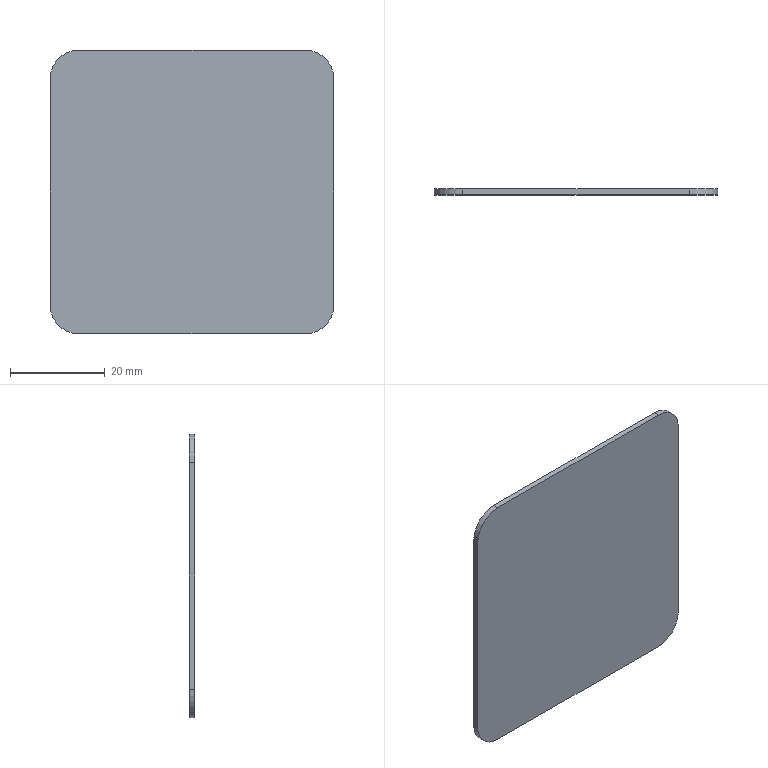Part | STEP file | JBJ-P-1017-02 | 1 solid | 10 faces | box 60 x 1.2 x 60 mm | volume 4283 mm3 | plane 6 | cylinder 4 | commonest cylinder face diameters 12 x4
STEP:
#1=CARTESIAN_POINT('',(30.,0.,-24.));
#2=VERTEX_POINT('',#1);
#3=CARTESIAN_POINT('',(24.,0.,-30.));
#4=VERTEX_POINT('',#3);
#5=CARTESIAN_POINT('',(24.,0.,-24.));
#6=DIRECTION('',(0.,1.,0.));
#7=DIRECTION('',(0.,0.,-1.));
#8=AXIS2_PLACEMENT_3D('',#5,#6,#7);
#9=CIRCLE('',#8,6.);
#10=EDGE_CURVE('',#2,#4,#9,.T.);
#11=ORIENTED_EDGE('',*,*,#10,.T.);
#12=CARTESIAN_POINT('',(24.,1.2,-30.));
#13=VERTEX_POINT('',#12);
#14=CARTESIAN_POINT('',(24.,1.2,-30.));
#15=DIRECTION('',(0.,-1.,0.));
#16=VECTOR('',#15,1000.);
#17=LINE('',#14,#16);
#18=EDGE_CURVE('',#13,#4,#17,.T.);
#19=ORIENTED_EDGE('',*,*,#18,.F.);
#20=CARTESIAN_POINT('',(30.,1.2,-24.));
#21=VERTEX_POINT('',#20);
#22=CARTESIAN_POINT('',(24.,1.2,-24.));
#23=DIRECTION('',(0.,1.,0.));
#24=DIRECTION('',(0.,0.,-1.));
#25=AXIS2_PLACEMENT_3D('',#22,#23,#24);
#26=CIRCLE('',#25,6.);
#27=EDGE_CURVE('',#21,#13,#26,.T.);
#28=ORIENTED_EDGE('',*,*,#27,.F.);
#29=CARTESIAN_POINT('',(30.,1.2,-24.));
#30=DIRECTION('',(0.,-1.,0.));
#31=VECTOR('',#30,1000.);
#32=LINE('',#29,#31);
#33=EDGE_CURVE('',#21,#2,#32,.T.);
#34=ORIENTED_EDGE('',*,*,#33,.T.);
#35=EDGE_LOOP('',(#11,#19,#28,#34));
#36=FACE_OUTER_BOUND('',#35,.T.);
#37=CARTESIAN_POINT('',(24.,1.2,-24.));
#38=DIRECTION('',(0.,-1.,0.));
#39=DIRECTION('',(0.,0.,-1.));
#40=AXIS2_PLACEMENT_3D('',#37,#38,#39);
#41=CYLINDRICAL_SURFACE('',#40,6.);
#42=ADVANCED_FACE('',(#36),#41,.T.);
#43=CARTESIAN_POINT('',(-24.,0.,-30.));
#44=VERTEX_POINT('',#43);
#45=CARTESIAN_POINT('',(-24.,0.,-30.));
#46=DIRECTION('',(-1.,0.,0.));
#47=VECTOR('',#46,1000.);
#48=LINE('',#45,#47);
#49=EDGE_CURVE('',#4,#44,#48,.T.);
#50=ORIENTED_EDGE('',*,*,#49,.T.);
#51=CARTESIAN_POINT('',(-24.,1.2,-30.));
#52=VERTEX_POINT('',#51);
#53=CARTESIAN_POINT('',(-24.,1.2,-30.));
#54=DIRECTION('',(0.,-1.,0.));
#55=VECTOR('',#54,1000.);
#56=LINE('',#53,#55);
#57=EDGE_CURVE('',#52,#44,#56,.T.);
#58=ORIENTED_EDGE('',*,*,#57,.F.);
#59=CARTESIAN_POINT('',(-24.,1.2,-30.));
#60=DIRECTION('',(-1.,0.,0.));
#61=VECTOR('',#60,1000.);
#62=LINE('',#59,#61);
#63=EDGE_CURVE('',#13,#52,#62,.T.);
#64=ORIENTED_EDGE('',*,*,#63,.F.);
#65=ORIENTED_EDGE('',*,*,#18,.T.);
#66=EDGE_LOOP('',(#50,#58,#64,#65));
#67=FACE_OUTER_BOUND('',#66,.T.);
#68=CARTESIAN_POINT('',(-24.,1.2,-30.));
#69=DIRECTION('',(0.,0.,1.));
#70=DIRECTION('',(1.,0.,0.));
#71=AXIS2_PLACEMENT_3D('',#68,#69,#70);
#72=PLANE('',#71);
#73=ADVANCED_FACE('',(#67),#72,.F.);
#74=CARTESIAN_POINT('',(-30.,0.,-24.));
#75=VERTEX_POINT('',#74);
#76=CARTESIAN_POINT('',(-24.,0.,-24.));
#77=DIRECTION('',(0.,1.,0.));
#78=DIRECTION('',(0.,0.,1.));
#79=AXIS2_PLACEMENT_3D('',#76,#77,#78);
#80=CIRCLE('',#79,6.);
#81=EDGE_CURVE('',#44,#75,#80,.T.);
#82=ORIENTED_EDGE('',*,*,#81,.T.);
#83=CARTESIAN_POINT('',(-30.,1.2,-24.));
#84=VERTEX_POINT('',#83);
#85=CARTESIAN_POINT('',(-30.,1.2,-24.));
#86=DIRECTION('',(0.,-1.,0.));
#87=VECTOR('',#86,1000.);
#88=LINE('',#85,#87);
#89=EDGE_CURVE('',#84,#75,#88,.T.);
#90=ORIENTED_EDGE('',*,*,#89,.F.);
#91=CARTESIAN_POINT('',(-24.,1.2,-24.));
#92=DIRECTION('',(0.,1.,0.));
#93=DIRECTION('',(0.,0.,1.));
#94=AXIS2_PLACEMENT_3D('',#91,#92,#93);
#95=CIRCLE('',#94,6.);
#96=EDGE_CURVE('',#52,#84,#95,.T.);
#97=ORIENTED_EDGE('',*,*,#96,.F.);
#98=ORIENTED_EDGE('',*,*,#57,.T.);
#99=EDGE_LOOP('',(#82,#90,#97,#98));
#100=FACE_OUTER_BOUND('',#99,.T.);
#101=CARTESIAN_POINT('',(-24.,1.2,-24.));
#102=DIRECTION('',(0.,-1.,0.));
#103=DIRECTION('',(0.,0.,-1.));
#104=AXIS2_PLACEMENT_3D('',#101,#102,#103);
#105=CYLINDRICAL_SURFACE('',#104,6.);
#106=ADVANCED_FACE('',(#100),#105,.T.);
#107=CARTESIAN_POINT('',(-30.,0.,24.));
#108=VERTEX_POINT('',#107);
#109=CARTESIAN_POINT('',(-30.,0.,-24.));
#110=DIRECTION('',(0.,0.,1.));
#111=VECTOR('',#110,1000.);
#112=LINE('',#109,#111);
#113=EDGE_CURVE('',#75,#108,#112,.T.);
#114=ORIENTED_EDGE('',*,*,#113,.T.);
#115=CARTESIAN_POINT('',(-30.,1.2,24.));
#116=VERTEX_POINT('',#115);
#117=CARTESIAN_POINT('',(-30.,1.2,24.));
#118=DIRECTION('',(0.,-1.,0.));
#119=VECTOR('',#118,1000.);
#120=LINE('',#117,#119);
#121=EDGE_CURVE('',#116,#108,#120,.T.);
#122=ORIENTED_EDGE('',*,*,#121,.F.);
#123=CARTESIAN_POINT('',(-30.,1.2,-24.));
#124=DIRECTION('',(0.,0.,1.));
#125=VECTOR('',#124,1000.);
#126=LINE('',#123,#125);
#127=EDGE_CURVE('',#84,#116,#126,.T.);
#128=ORIENTED_EDGE('',*,*,#127,.F.);
#129=ORIENTED_EDGE('',*,*,#89,.T.);
#130=EDGE_LOOP('',(#114,#122,#128,#129));
#131=FACE_OUTER_BOUND('',#130,.T.);
#132=CARTESIAN_POINT('',(-30.,1.2,-24.));
#133=DIRECTION('',(1.,0.,0.));
#134=DIRECTION('',(0.,0.,-1.));
#135=AXIS2_PLACEMENT_3D('',#132,#133,#134);
#136=PLANE('',#135);
#137=ADVANCED_FACE('',(#131),#136,.F.);
#138=CARTESIAN_POINT('',(-24.,0.,30.));
#139=VERTEX_POINT('',#138);
#140=CARTESIAN_POINT('',(-24.,0.,24.));
#141=DIRECTION('',(0.,1.,0.));
#142=DIRECTION('',(0.,0.,1.));
#143=AXIS2_PLACEMENT_3D('',#140,#141,#142);
#144=CIRCLE('',#143,6.);
#145=EDGE_CURVE('',#108,#139,#144,.T.);
#146=ORIENTED_EDGE('',*,*,#145,.T.);
#147=CARTESIAN_POINT('',(-24.,1.2,30.));
#148=VERTEX_POINT('',#147);
#149=CARTESIAN_POINT('',(-24.,1.2,30.));
#150=DIRECTION('',(0.,-1.,0.));
#151=VECTOR('',#150,1000.);
#152=LINE('',#149,#151);
#153=EDGE_CURVE('',#148,#139,#152,.T.);
#154=ORIENTED_EDGE('',*,*,#153,.F.);
#155=CARTESIAN_POINT('',(-24.,1.2,24.));
#156=DIRECTION('',(0.,1.,0.));
#157=DIRECTION('',(0.,0.,1.));
#158=AXIS2_PLACEMENT_3D('',#155,#156,#157);
#159=CIRCLE('',#158,6.);
#160=EDGE_CURVE('',#116,#148,#159,.T.);
#161=ORIENTED_EDGE('',*,*,#160,.F.);
#162=ORIENTED_EDGE('',*,*,#121,.T.);
#163=EDGE_LOOP('',(#146,#154,#161,#162));
#164=FACE_OUTER_BOUND('',#163,.T.);
#165=CARTESIAN_POINT('',(-24.,1.2,24.));
#166=DIRECTION('',(0.,-1.,0.));
#167=DIRECTION('',(0.,0.,-1.));
#168=AXIS2_PLACEMENT_3D('',#165,#166,#167);
#169=CYLINDRICAL_SURFACE('',#168,6.);
#170=ADVANCED_FACE('',(#164),#169,.T.);
#171=CARTESIAN_POINT('',(24.,0.,30.));
#172=VERTEX_POINT('',#171);
#173=CARTESIAN_POINT('',(-24.,0.,30.));
#174=DIRECTION('',(1.,0.,0.));
#175=VECTOR('',#174,1000.);
#176=LINE('',#173,#175);
#177=EDGE_CURVE('',#139,#172,#176,.T.);
#178=ORIENTED_EDGE('',*,*,#177,.T.);
#179=CARTESIAN_POINT('',(24.,1.2,30.));
#180=VERTEX_POINT('',#179);
#181=CARTESIAN_POINT('',(24.,1.2,30.));
#182=DIRECTION('',(0.,-1.,0.));
#183=VECTOR('',#182,1000.);
#184=LINE('',#181,#183);
#185=EDGE_CURVE('',#180,#172,#184,.T.);
#186=ORIENTED_EDGE('',*,*,#185,.F.);
#187=CARTESIAN_POINT('',(-24.,1.2,30.));
#188=DIRECTION('',(1.,0.,0.));
#189=VECTOR('',#188,1000.);
#190=LINE('',#187,#189);
#191=EDGE_CURVE('',#148,#180,#190,.T.);
#192=ORIENTED_EDGE('',*,*,#191,.F.);
#193=ORIENTED_EDGE('',*,*,#153,.T.);
#194=EDGE_LOOP('',(#178,#186,#192,#193));
#195=FACE_OUTER_BOUND('',#194,.T.);
#196=CARTESIAN_POINT('',(-24.,1.2,30.));
#197=DIRECTION('',(0.,0.,-1.));
#198=DIRECTION('',(-1.,0.,0.));
#199=AXIS2_PLACEMENT_3D('',#196,#197,#198);
#200=PLANE('',#199);
#201=ADVANCED_FACE('',(#195),#200,.F.);
#202=CARTESIAN_POINT('',(30.,0.,24.));
#203=VERTEX_POINT('',#202);
#204=CARTESIAN_POINT('',(24.,0.,24.));
#205=DIRECTION('',(0.,1.,0.));
#206=DIRECTION('',(0.,0.,1.));
#207=AXIS2_PLACEMENT_3D('',#204,#205,#206);
#208=CIRCLE('',#207,6.);
#209=EDGE_CURVE('',#172,#203,#208,.T.);
#210=ORIENTED_EDGE('',*,*,#209,.T.);
#211=CARTESIAN_POINT('',(30.,1.2,24.));
#212=VERTEX_POINT('',#211);
#213=CARTESIAN_POINT('',(30.,1.2,24.));
#214=DIRECTION('',(0.,-1.,0.));
#215=VECTOR('',#214,1000.);
#216=LINE('',#213,#215);
#217=EDGE_CURVE('',#212,#203,#216,.T.);
#218=ORIENTED_EDGE('',*,*,#217,.F.);
#219=CARTESIAN_POINT('',(24.,1.2,24.));
#220=DIRECTION('',(0.,1.,0.));
#221=DIRECTION('',(0.,0.,1.));
#222=AXIS2_PLACEMENT_3D('',#219,#220,#221);
#223=CIRCLE('',#222,6.);
#224=EDGE_CURVE('',#180,#212,#223,.T.);
#225=ORIENTED_EDGE('',*,*,#224,.F.);
#226=ORIENTED_EDGE('',*,*,#185,.T.);
#227=EDGE_LOOP('',(#210,#218,#225,#226));
#228=FACE_OUTER_BOUND('',#227,.T.);
#229=CARTESIAN_POINT('',(24.,1.2,24.));
#230=DIRECTION('',(0.,-1.,0.));
#231=DIRECTION('',(0.,0.,-1.));
#232=AXIS2_PLACEMENT_3D('',#229,#230,#231);
#233=CYLINDRICAL_SURFACE('',#232,6.);
#234=ADVANCED_FACE('',(#228),#233,.T.);
#235=CARTESIAN_POINT('',(30.,0.,-24.));
#236=DIRECTION('',(0.,0.,-1.));
#237=VECTOR('',#236,1000.);
#238=LINE('',#235,#237);
#239=EDGE_CURVE('',#203,#2,#238,.T.);
#240=ORIENTED_EDGE('',*,*,#239,.T.);
#241=ORIENTED_EDGE('',*,*,#33,.F.);
#242=CARTESIAN_POINT('',(30.,1.2,-24.));
#243=DIRECTION('',(0.,0.,-1.));
#244=VECTOR('',#243,1000.);
#245=LINE('',#242,#244);
#246=EDGE_CURVE('',#212,#21,#245,.T.);
#247=ORIENTED_EDGE('',*,*,#246,.F.);
#248=ORIENTED_EDGE('',*,*,#217,.T.);
#249=EDGE_LOOP('',(#240,#241,#247,#248));
#250=FACE_OUTER_BOUND('',#249,.T.);
#251=CARTESIAN_POINT('',(30.,1.2,-24.));
#252=DIRECTION('',(-1.,0.,0.));
#253=DIRECTION('',(0.,0.,1.));
#254=AXIS2_PLACEMENT_3D('',#251,#252,#253);
#255=PLANE('',#254);
#256=ADVANCED_FACE('',(#250),#255,.F.);
#257=ORIENTED_EDGE('',*,*,#27,.T.);
#258=ORIENTED_EDGE('',*,*,#63,.T.);
#259=ORIENTED_EDGE('',*,*,#96,.T.);
#260=ORIENTED_EDGE('',*,*,#127,.T.);
#261=ORIENTED_EDGE('',*,*,#160,.T.);
#262=ORIENTED_EDGE('',*,*,#191,.T.);
#263=ORIENTED_EDGE('',*,*,#224,.T.);
#264=ORIENTED_EDGE('',*,*,#246,.T.);
#265=EDGE_LOOP('',(#257,#258,#259,#260,#261,#262,#263,#264));
#266=FACE_OUTER_BOUND('',#265,.T.);
#267=CARTESIAN_POINT('',(24.,1.2,-24.));
#268=DIRECTION('',(0.,-1.,0.));
#269=DIRECTION('',(0.,0.,-1.));
#270=AXIS2_PLACEMENT_3D('',#267,#268,#269);
#271=PLANE('',#270);
#272=ADVANCED_FACE('',(#266),#271,.F.);
#273=ORIENTED_EDGE('',*,*,#10,.F.);
#274=ORIENTED_EDGE('',*,*,#239,.F.);
#275=ORIENTED_EDGE('',*,*,#209,.F.);
#276=ORIENTED_EDGE('',*,*,#177,.F.);
#277=ORIENTED_EDGE('',*,*,#145,.F.);
#278=ORIENTED_EDGE('',*,*,#113,.F.);
#279=ORIENTED_EDGE('',*,*,#81,.F.);
#280=ORIENTED_EDGE('',*,*,#49,.F.);
#281=EDGE_LOOP('',(#273,#274,#275,#276,#277,#278,#279,#280));
#282=FACE_OUTER_BOUND('',#281,.T.);
#283=CARTESIAN_POINT('',(24.,0.,-24.));
#284=DIRECTION('',(0.,-1.,0.));
#285=DIRECTION('',(0.,0.,-1.));
#286=AXIS2_PLACEMENT_3D('',#283,#284,#285);
#287=PLANE('',#286);
#288=ADVANCED_FACE('',(#282),#287,.T.);
#289=CLOSED_SHELL('',(#42,#73,#106,#137,#170,#201,#234,#256,#272,#288));
#290=MANIFOLD_SOLID_BREP('',#289);
#291=CARTESIAN_POINT('',(0.,0.,0.));
#292=DIRECTION('',(0.,0.,1.));
#293=DIRECTION('',(1.,0.,0.));
#294=AXIS2_PLACEMENT_3D('',#291,#292,#293);
#295=(LENGTH_UNIT()NAMED_UNIT(*)SI_UNIT(.MILLI.,.METRE.));
#296=UNCERTAINTY_MEASURE_WITH_UNIT(LENGTH_MEASURE(0.00001),#295,'','');
#297=(NAMED_UNIT(*)PLANE_ANGLE_UNIT()SI_UNIT($,.RADIAN.));
#298=(NAMED_UNIT(*)SI_UNIT($,.STERADIAN.)SOLID_ANGLE_UNIT());
#299=(GEOMETRIC_REPRESENTATION_CONTEXT(3)GLOBAL_UNCERTAINTY_ASSIGNED_CONTEXT((#296))GLOBAL_UNIT_ASSIGNED_CONTEXT((#295,#297,#298))REPRESENTATION_CONTEXT('',''));
#300=ADVANCED_BREP_SHAPE_REPRESENTATION('',(#290,#294),#299);